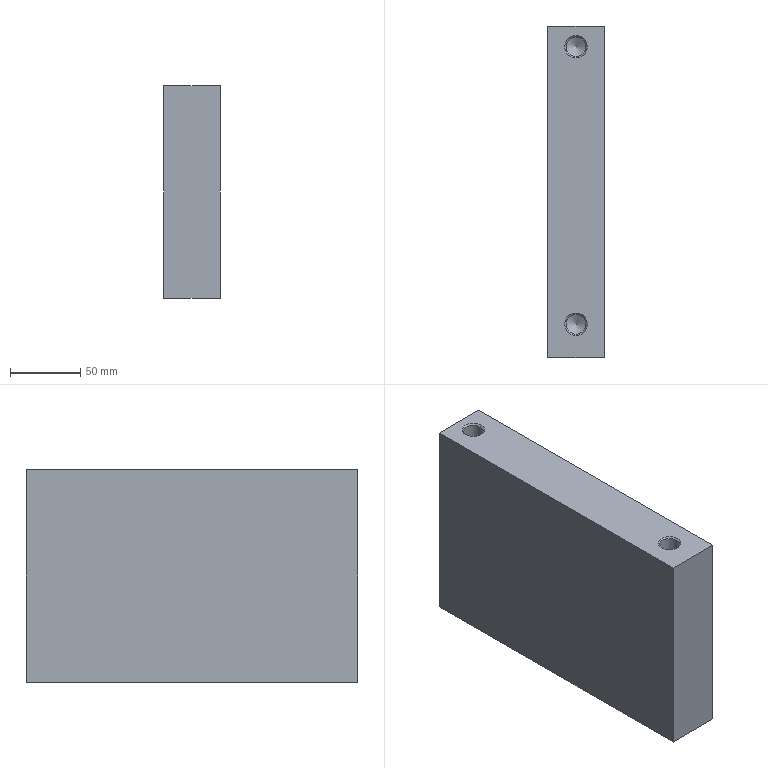Part | NX | features solid 2 | 1 solid | 15 faces | box 40 x 235 x 151.131 mm | volume 1399130 mm3 | plane 6 | cone 6 | cylinder 3 | commonest cylinder face diameters 14 x3
STEP:
#1=CARTESIAN_POINT('',(1529.977,-352.905,246.13));
#2=VERTEX_POINT('',#1);
#3=CARTESIAN_POINT('',(1569.977,-352.905,246.13));
#4=VERTEX_POINT('',#3);
#5=CARTESIAN_POINT('',(1344.977,-352.905,246.13));
#6=DIRECTION('',(1.,0.,0.));
#7=VECTOR('',#6,1000.);
#8=LINE('',#5,#7);
#9=EDGE_CURVE('',#2,#4,#8,.T.);
#10=ORIENTED_EDGE('',*,*,#9,.F.);
#11=CARTESIAN_POINT('',(1529.977,-352.905,94.999));
#12=VERTEX_POINT('',#11);
#13=CARTESIAN_POINT('',(1529.977,-352.905,289.999));
#14=DIRECTION('',(0.,0.,-1.));
#15=VECTOR('',#14,1000.);
#16=LINE('',#13,#15);
#17=EDGE_CURVE('',#2,#12,#16,.T.);
#18=ORIENTED_EDGE('',*,*,#17,.T.);
#19=CARTESIAN_POINT('',(1569.977,-352.905,94.999));
#20=VERTEX_POINT('',#19);
#21=CARTESIAN_POINT('',(1344.977,-352.905,94.999));
#22=DIRECTION('',(1.,0.,0.));
#23=VECTOR('',#22,1000.);
#24=LINE('',#21,#23);
#25=EDGE_CURVE('',#20,#12,#24,.F.);
#26=ORIENTED_EDGE('',*,*,#25,.F.);
#27=CARTESIAN_POINT('',(1569.977,-352.905,159.999));
#28=DIRECTION('',(0.,0.,-1.));
#29=VECTOR('',#28,1000.);
#30=LINE('',#27,#29);
#31=EDGE_CURVE('',#4,#20,#30,.T.);
#32=ORIENTED_EDGE('',*,*,#31,.F.);
#33=EDGE_LOOP('',(#10,#18,#26,#32));
#34=FACE_BOUND('',#33,.T.);
#35=CARTESIAN_POINT('',(1344.977,-352.905,289.999));
#36=DIRECTION('',(0.,-1.,0.));
#37=DIRECTION('',(0.,0.,-1.));
#38=AXIS2_PLACEMENT_3D('',#35,#36,#37);
#39=PLANE('',#38);
#40=ADVANCED_FACE('',(#34),#39,.T.);
#41=CARTESIAN_POINT('',(1541.977,-132.405,246.13));
#42=VERTEX_POINT('',#41);
#43=CARTESIAN_POINT('',(1549.977,-132.405,246.13));
#44=DIRECTION('',(0.,0.,-1.));
#45=DIRECTION('',(-1.,0.,0.));
#46=AXIS2_PLACEMENT_3D('',#43,#44,#45);
#47=CIRCLE('',#46,8.);
#48=EDGE_CURVE('',#42,#42,#47,.T.);
#49=ORIENTED_EDGE('',*,*,#48,.T.);
#50=EDGE_LOOP('',(#49));
#51=FACE_BOUND('',#50,.T.);
#52=CARTESIAN_POINT('',(1541.977,-329.405,246.13));
#53=VERTEX_POINT('',#52);
#54=CARTESIAN_POINT('',(1549.977,-329.405,246.13));
#55=DIRECTION('',(0.,0.,-1.));
#56=DIRECTION('',(-1.,0.,0.));
#57=AXIS2_PLACEMENT_3D('',#54,#55,#56);
#58=CIRCLE('',#57,8.);
#59=EDGE_CURVE('',#53,#53,#58,.T.);
#60=ORIENTED_EDGE('',*,*,#59,.T.);
#61=EDGE_LOOP('',(#60));
#62=FACE_BOUND('',#61,.T.);
#63=CARTESIAN_POINT('',(1569.977,-117.905,246.13));
#64=VERTEX_POINT('',#63);
#65=CARTESIAN_POINT('',(1569.977,4.191,246.13));
#66=DIRECTION('',(0.,-1.,0.));
#67=VECTOR('',#66,1000.);
#68=LINE('',#65,#67);
#69=EDGE_CURVE('',#64,#4,#68,.T.);
#70=ORIENTED_EDGE('',*,*,#69,.F.);
#71=CARTESIAN_POINT('',(1529.977,-117.905,246.13));
#72=VERTEX_POINT('',#71);
#73=CARTESIAN_POINT('',(1540.977,-117.905,246.13));
#74=DIRECTION('',(1.,0.,0.));
#75=VECTOR('',#74,1000.);
#76=LINE('',#73,#75);
#77=EDGE_CURVE('',#72,#64,#76,.T.);
#78=ORIENTED_EDGE('',*,*,#77,.F.);
#79=CARTESIAN_POINT('',(1529.977,4.191,246.13));
#80=DIRECTION('',(0.,1.,0.));
#81=VECTOR('',#80,1000.);
#82=LINE('',#79,#81);
#83=EDGE_CURVE('',#2,#72,#82,.T.);
#84=ORIENTED_EDGE('',*,*,#83,.F.);
#85=ORIENTED_EDGE('',*,*,#9,.T.);
#86=EDGE_LOOP('',(#70,#78,#84,#85));
#87=FACE_BOUND('',#86,.T.);
#88=CARTESIAN_POINT('',(3499.955,4.191,246.13));
#89=DIRECTION('',(0.,0.,-1.));
#90=DIRECTION('',(1.,0.,0.));
#91=AXIS2_PLACEMENT_3D('',#88,#89,#90);
#92=PLANE('',#91);
#93=ADVANCED_FACE('',(#51,#62,#87),#92,.F.);
#94=CARTESIAN_POINT('',(1541.977,-329.405,94.999));
#95=VERTEX_POINT('',#94);
#96=CARTESIAN_POINT('',(1549.977,-329.405,94.999));
#97=DIRECTION('',(0.,0.,-1.));
#98=DIRECTION('',(-1.,0.,0.));
#99=AXIS2_PLACEMENT_3D('',#96,#97,#98);
#100=CIRCLE('',#99,8.);
#101=EDGE_CURVE('',#95,#95,#100,.F.);
#102=ORIENTED_EDGE('',*,*,#101,.T.);
#103=EDGE_LOOP('',(#102));
#104=FACE_BOUND('',#103,.T.);
#105=CARTESIAN_POINT('',(1529.977,-117.905,94.999));
#106=VERTEX_POINT('',#105);
#107=CARTESIAN_POINT('',(1529.977,6.94,94.999));
#108=DIRECTION('',(0.,-1.,0.));
#109=VECTOR('',#108,1000.);
#110=LINE('',#107,#109);
#111=EDGE_CURVE('',#12,#106,#110,.F.);
#112=ORIENTED_EDGE('',*,*,#111,.T.);
#113=CARTESIAN_POINT('',(1569.977,-117.905,94.999));
#114=VERTEX_POINT('',#113);
#115=CARTESIAN_POINT('',(1364.955,-117.905,94.999));
#116=DIRECTION('',(-1.,0.,0.));
#117=VECTOR('',#116,1000.);
#118=LINE('',#115,#117);
#119=EDGE_CURVE('',#106,#114,#118,.F.);
#120=ORIENTED_EDGE('',*,*,#119,.T.);
#121=CARTESIAN_POINT('',(1569.977,6.94,94.999));
#122=DIRECTION('',(0.,1.,0.));
#123=VECTOR('',#122,1000.);
#124=LINE('',#121,#123);
#125=EDGE_CURVE('',#114,#20,#124,.F.);
#126=ORIENTED_EDGE('',*,*,#125,.T.);
#127=ORIENTED_EDGE('',*,*,#25,.T.);
#128=EDGE_LOOP('',(#112,#120,#126,#127));
#129=FACE_BOUND('',#128,.T.);
#130=CARTESIAN_POINT('',(1364.955,6.94,94.999));
#131=DIRECTION('',(0.,0.,-1.));
#132=DIRECTION('',(-1.,0.,0.));
#133=AXIS2_PLACEMENT_3D('',#130,#131,#132);
#134=PLANE('',#133);
#135=ADVANCED_FACE('',(#104,#129),#134,.T.);
#136=CARTESIAN_POINT('',(1529.977,-117.905,159.999));
#137=DIRECTION('',(0.,0.,1.));
#138=VECTOR('',#137,1000.);
#139=LINE('',#136,#138);
#140=EDGE_CURVE('',#106,#72,#139,.T.);
#141=ORIENTED_EDGE('',*,*,#140,.F.);
#142=ORIENTED_EDGE('',*,*,#111,.F.);
#143=ORIENTED_EDGE('',*,*,#17,.F.);
#144=ORIENTED_EDGE('',*,*,#83,.T.);
#145=EDGE_LOOP('',(#141,#142,#143,#144));
#146=FACE_BOUND('',#145,.T.);
#147=CARTESIAN_POINT('',(1529.977,2.095,159.999));
#148=DIRECTION('',(-1.,0.,0.));
#149=DIRECTION('',(0.,0.,1.));
#150=AXIS2_PLACEMENT_3D('',#147,#148,#149);
#151=PLANE('',#150);
#152=ADVANCED_FACE('',(#146),#151,.T.);
#153=CARTESIAN_POINT('',(1569.977,-117.905,159.999));
#154=DIRECTION('',(0.,0.,-1.));
#155=VECTOR('',#154,1000.);
#156=LINE('',#153,#155);
#157=EDGE_CURVE('',#64,#114,#156,.T.);
#158=ORIENTED_EDGE('',*,*,#157,.F.);
#159=ORIENTED_EDGE('',*,*,#69,.T.);
#160=ORIENTED_EDGE('',*,*,#31,.T.);
#161=ORIENTED_EDGE('',*,*,#125,.F.);
#162=EDGE_LOOP('',(#158,#159,#160,#161));
#163=FACE_BOUND('',#162,.T.);
#164=CARTESIAN_POINT('',(1569.977,2.095,159.999));
#165=DIRECTION('',(1.,0.,0.));
#166=DIRECTION('',(0.,0.,-1.));
#167=AXIS2_PLACEMENT_3D('',#164,#165,#166);
#168=PLANE('',#167);
#169=ADVANCED_FACE('',(#163),#168,.T.);
#170=ORIENTED_EDGE('',*,*,#140,.T.);
#171=ORIENTED_EDGE('',*,*,#77,.T.);
#172=ORIENTED_EDGE('',*,*,#157,.T.);
#173=ORIENTED_EDGE('',*,*,#119,.F.);
#174=EDGE_LOOP('',(#170,#171,#172,#173));
#175=FACE_BOUND('',#174,.T.);
#176=CARTESIAN_POINT('',(1540.977,-117.905,149.065));
#177=DIRECTION('',(0.,-1.,0.));
#178=DIRECTION('',(0.,0.,1.));
#179=AXIS2_PLACEMENT_3D('',#176,#177,#178);
#180=PLANE('',#179);
#181=ADVANCED_FACE('',(#175),#180,.F.);
#182=CARTESIAN_POINT('',(1542.977,-329.405,201.13));
#183=VERTEX_POINT('',#182);
#184=CARTESIAN_POINT('',(1549.977,-329.405,201.13));
#185=DIRECTION('',(0.,0.,-1.));
#186=DIRECTION('',(-1.,0.,0.));
#187=AXIS2_PLACEMENT_3D('',#184,#185,#186);
#188=CIRCLE('',#187,7.);
#189=EDGE_CURVE('',#183,#183,#188,.F.);
#190=ORIENTED_EDGE('',*,*,#189,.T.);
#191=EDGE_LOOP('',(#190));
#192=FACE_BOUND('',#191,.T.);
#193=CARTESIAN_POINT('',(1549.977,-329.405,196.924));
#194=VERTEX_POINT('',#193);
#195=VERTEX_LOOP('',#194);
#196=FACE_BOUND('',#195,.T.);
#197=CARTESIAN_POINT('',(1549.977,-329.405,201.13));
#198=DIRECTION('',(0.,0.,1.));
#199=DIRECTION('',(1.,0.,0.));
#200=AXIS2_PLACEMENT_3D('',#197,#198,#199);
#201=CONICAL_SURFACE('',#200,7.,1.03);
#202=ADVANCED_FACE('',(#192,#196),#201,.F.);
#203=CARTESIAN_POINT('',(1542.977,-329.405,245.13));
#204=VERTEX_POINT('',#203);
#205=CARTESIAN_POINT('',(1549.977,-329.405,245.13));
#206=DIRECTION('',(0.,0.,-1.));
#207=DIRECTION('',(-1.,0.,0.));
#208=AXIS2_PLACEMENT_3D('',#205,#206,#207);
#209=CIRCLE('',#208,7.);
#210=EDGE_CURVE('',#204,#204,#209,.F.);
#211=ORIENTED_EDGE('',*,*,#210,.T.);
#212=EDGE_LOOP('',(#211));
#213=FACE_BOUND('',#212,.T.);
#214=ORIENTED_EDGE('',*,*,#189,.F.);
#215=EDGE_LOOP('',(#214));
#216=FACE_BOUND('',#215,.T.);
#217=CARTESIAN_POINT('',(1549.977,-329.405,246.13));
#218=DIRECTION('',(0.,0.,-1.));
#219=DIRECTION('',(-1.,0.,0.));
#220=AXIS2_PLACEMENT_3D('',#217,#218,#219);
#221=CYLINDRICAL_SURFACE('',#220,7.);
#222=ADVANCED_FACE('',(#213,#216),#221,.F.);
#223=ORIENTED_EDGE('',*,*,#210,.F.);
#224=EDGE_LOOP('',(#223));
#225=FACE_BOUND('',#224,.T.);
#226=ORIENTED_EDGE('',*,*,#59,.F.);
#227=EDGE_LOOP('',(#226));
#228=FACE_BOUND('',#227,.T.);
#229=CARTESIAN_POINT('',(1549.977,-329.405,246.13));
#230=DIRECTION('',(0.,0.,1.));
#231=DIRECTION('',(1.,0.,0.));
#232=AXIS2_PLACEMENT_3D('',#229,#230,#231);
#233=CONICAL_SURFACE('',#232,8.,0.7854);
#234=ADVANCED_FACE('',(#225,#228),#233,.F.);
#235=CARTESIAN_POINT('',(1542.977,-132.405,201.13));
#236=VERTEX_POINT('',#235);
#237=CARTESIAN_POINT('',(1549.977,-132.405,201.13));
#238=DIRECTION('',(0.,0.,-1.));
#239=DIRECTION('',(-1.,0.,0.));
#240=AXIS2_PLACEMENT_3D('',#237,#238,#239);
#241=CIRCLE('',#240,7.);
#242=EDGE_CURVE('',#236,#236,#241,.F.);
#243=ORIENTED_EDGE('',*,*,#242,.T.);
#244=EDGE_LOOP('',(#243));
#245=FACE_BOUND('',#244,.T.);
#246=CARTESIAN_POINT('',(1549.977,-132.405,196.924));
#247=VERTEX_POINT('',#246);
#248=VERTEX_LOOP('',#247);
#249=FACE_BOUND('',#248,.T.);
#250=CARTESIAN_POINT('',(1549.977,-132.405,201.13));
#251=DIRECTION('',(0.,0.,1.));
#252=DIRECTION('',(1.,0.,0.));
#253=AXIS2_PLACEMENT_3D('',#250,#251,#252);
#254=CONICAL_SURFACE('',#253,7.,1.03);
#255=ADVANCED_FACE('',(#245,#249),#254,.F.);
#256=CARTESIAN_POINT('',(1542.977,-132.405,245.13));
#257=VERTEX_POINT('',#256);
#258=CARTESIAN_POINT('',(1549.977,-132.405,245.13));
#259=DIRECTION('',(0.,0.,-1.));
#260=DIRECTION('',(-1.,0.,0.));
#261=AXIS2_PLACEMENT_3D('',#258,#259,#260);
#262=CIRCLE('',#261,7.);
#263=EDGE_CURVE('',#257,#257,#262,.F.);
#264=ORIENTED_EDGE('',*,*,#263,.T.);
#265=EDGE_LOOP('',(#264));
#266=FACE_BOUND('',#265,.T.);
#267=ORIENTED_EDGE('',*,*,#242,.F.);
#268=EDGE_LOOP('',(#267));
#269=FACE_BOUND('',#268,.T.);
#270=CARTESIAN_POINT('',(1549.977,-132.405,246.13));
#271=DIRECTION('',(0.,0.,-1.));
#272=DIRECTION('',(-1.,0.,0.));
#273=AXIS2_PLACEMENT_3D('',#270,#271,#272);
#274=CYLINDRICAL_SURFACE('',#273,7.);
#275=ADVANCED_FACE('',(#266,#269),#274,.F.);
#276=ORIENTED_EDGE('',*,*,#263,.F.);
#277=EDGE_LOOP('',(#276));
#278=FACE_BOUND('',#277,.T.);
#279=ORIENTED_EDGE('',*,*,#48,.F.);
#280=EDGE_LOOP('',(#279));
#281=FACE_BOUND('',#280,.T.);
#282=CARTESIAN_POINT('',(1549.977,-132.405,246.13));
#283=DIRECTION('',(0.,0.,1.));
#284=DIRECTION('',(1.,0.,0.));
#285=AXIS2_PLACEMENT_3D('',#282,#283,#284);
#286=CONICAL_SURFACE('',#285,8.,0.7854);
#287=ADVANCED_FACE('',(#278,#281),#286,.F.);
#288=CARTESIAN_POINT('',(1556.977,-329.405,139.999));
#289=VERTEX_POINT('',#288);
#290=CARTESIAN_POINT('',(1549.977,-329.405,139.999));
#291=DIRECTION('',(0.,0.,1.));
#292=DIRECTION('',(1.,0.,0.));
#293=AXIS2_PLACEMENT_3D('',#290,#291,#292);
#294=CIRCLE('',#293,7.);
#295=EDGE_CURVE('',#289,#289,#294,.F.);
#296=ORIENTED_EDGE('',*,*,#295,.T.);
#297=EDGE_LOOP('',(#296));
#298=FACE_BOUND('',#297,.T.);
#299=CARTESIAN_POINT('',(1549.977,-329.405,144.205));
#300=VERTEX_POINT('',#299);
#301=VERTEX_LOOP('',#300);
#302=FACE_BOUND('',#301,.T.);
#303=CARTESIAN_POINT('',(1549.977,-329.405,139.999));
#304=DIRECTION('',(0.,0.,-1.));
#305=DIRECTION('',(-1.,0.,0.));
#306=AXIS2_PLACEMENT_3D('',#303,#304,#305);
#307=CONICAL_SURFACE('',#306,7.,1.03);
#308=ADVANCED_FACE('',(#298,#302),#307,.F.);
#309=CARTESIAN_POINT('',(1556.977,-329.405,95.999));
#310=VERTEX_POINT('',#309);
#311=CARTESIAN_POINT('',(1549.977,-329.405,95.999));
#312=DIRECTION('',(0.,0.,1.));
#313=DIRECTION('',(1.,0.,0.));
#314=AXIS2_PLACEMENT_3D('',#311,#312,#313);
#315=CIRCLE('',#314,7.);
#316=EDGE_CURVE('',#310,#310,#315,.F.);
#317=ORIENTED_EDGE('',*,*,#316,.T.);
#318=EDGE_LOOP('',(#317));
#319=FACE_BOUND('',#318,.T.);
#320=ORIENTED_EDGE('',*,*,#295,.F.);
#321=EDGE_LOOP('',(#320));
#322=FACE_BOUND('',#321,.T.);
#323=CARTESIAN_POINT('',(1549.977,-329.405,94.999));
#324=DIRECTION('',(0.,0.,1.));
#325=DIRECTION('',(1.,0.,0.));
#326=AXIS2_PLACEMENT_3D('',#323,#324,#325);
#327=CYLINDRICAL_SURFACE('',#326,7.);
#328=ADVANCED_FACE('',(#319,#322),#327,.F.);
#329=ORIENTED_EDGE('',*,*,#316,.F.);
#330=EDGE_LOOP('',(#329));
#331=FACE_BOUND('',#330,.T.);
#332=ORIENTED_EDGE('',*,*,#101,.F.);
#333=EDGE_LOOP('',(#332));
#334=FACE_BOUND('',#333,.T.);
#335=CARTESIAN_POINT('',(1549.977,-329.405,94.999));
#336=DIRECTION('',(0.,0.,-1.));
#337=DIRECTION('',(-1.,0.,0.));
#338=AXIS2_PLACEMENT_3D('',#335,#336,#337);
#339=CONICAL_SURFACE('',#338,8.,0.7854);
#340=ADVANCED_FACE('',(#331,#334),#339,.F.);
#341=CLOSED_SHELL('',(#40,#93,#135,#152,#169,#181,#202,#222,#234,#255,#275,#287,#308,#328,#340));
#342=MANIFOLD_SOLID_BREP('',#341);
#343=(LENGTH_UNIT()NAMED_UNIT(*)SI_UNIT(.MILLI.,.METRE.));
#344=UNCERTAINTY_MEASURE_WITH_UNIT(LENGTH_MEASURE(0.00001),#343,'','');
#345=(NAMED_UNIT(*)PLANE_ANGLE_UNIT()SI_UNIT($,.RADIAN.));
#346=(NAMED_UNIT(*)SI_UNIT($,.STERADIAN.)SOLID_ANGLE_UNIT());
#347=(GEOMETRIC_REPRESENTATION_CONTEXT(3)GLOBAL_UNCERTAINTY_ASSIGNED_CONTEXT((#344))GLOBAL_UNIT_ASSIGNED_CONTEXT((#343,#345,#346))REPRESENTATION_CONTEXT('',''));
#348=ADVANCED_BREP_SHAPE_REPRESENTATION('',(#342),#347);